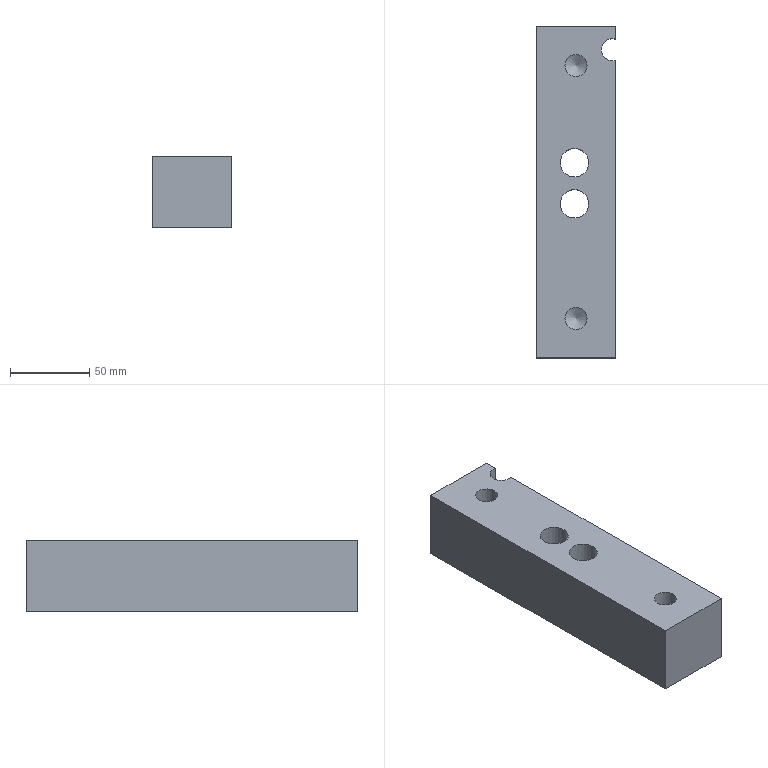Part | STEP file | 012_id2190_x_t | 1 solid | 14 faces | box 50 x 210 x 45 mm | volume 438486 mm3 | plane 7 | cylinder 5 | cone 2 | commonest cylinder face diameters 14 x3 18 x2
STEP:
#1=CARTESIAN_POINT('',(0.,0.,0.));
#2=DIRECTION('',(0.,0.,1.));
#3=DIRECTION('',(1.,0.,0.));
#4=AXIS2_PLACEMENT_3D('',#1,#2,#3);
#5=CARTESIAN_POINT('',(-853.5,103.5,230.));
#6=VERTEX_POINT('',#5);
#7=CARTESIAN_POINT('',(-862.5,103.5,230.));
#8=DIRECTION('',(0.,0.,-1.));
#9=DIRECTION('',(1.,0.,0.));
#10=AXIS2_PLACEMENT_3D('',#7,#8,#9);
#11=CIRCLE('',#10,9.);
#12=CARTESIAN_POINT('',(-681.5,-210.,230.));
#13=DIRECTION('',(0.,0.,1.));
#14=DIRECTION('',(1.,0.,0.));
#15=AXIS2_PLACEMENT_3D('',#12,#13,#14);
#16=PLANE('',#15);
#17=CARTESIAN_POINT('',(-172.,313.5));
#18=CARTESIAN_POINT('',(-172.,297.912));
#19=CARTESIAN_POINT('',(-185.5,305.706));
#20=CARTESIAN_POINT('',(-199.,313.5));
#21=CARTESIAN_POINT('',(-185.5,321.294));
#22=CARTESIAN_POINT('',(-172.,329.088));
#23=CARTESIAN_POINT('',(-172.,313.5));
#24=(BOUNDED_CURVE()B_SPLINE_CURVE(2,(#17,#18,#19,#20,#21,#22,#23),.UNSPECIFIED.,.T.,.F.)B_SPLINE_CURVE_WITH_KNOTS((1,2,2,2,2,1),(-2.094,0.,2.094,4.189,6.283,8.378),.UNSPECIFIED.)CURVE()GEOMETRIC_REPRESENTATION_ITEM()RATIONAL_B_SPLINE_CURVE((1.,0.5,1.,0.5,1.,0.5,1.))REPRESENTATION_ITEM(''));
#25=(GEOMETRIC_REPRESENTATION_CONTEXT(2)PARAMETRIC_REPRESENTATION_CONTEXT()REPRESENTATION_CONTEXT('',''));
#26=DEFINITIONAL_REPRESENTATION('',(#24),#25);
#27=PCURVE('',#16,#26);
#28=CARTESIAN_POINT('',(-862.5,103.5,510.));
#29=DIRECTION('',(0.,0.,-1.));
#30=DIRECTION('',(-1.,0.,0.));
#31=AXIS2_PLACEMENT_3D('',#28,#29,#30);
#32=CYLINDRICAL_SURFACE('',#31,9.);
#33=CARTESIAN_POINT('',(3.142,280.));
#34=DIRECTION('',(1.,0.));
#35=VECTOR('',#34,1.);
#36=LINE('',#33,#35);
#37=(GEOMETRIC_REPRESENTATION_CONTEXT(2)PARAMETRIC_REPRESENTATION_CONTEXT()REPRESENTATION_CONTEXT('',''));
#38=DEFINITIONAL_REPRESENTATION('',(#36),#37);
#39=PCURVE('',#32,#38);
#40=SURFACE_CURVE('',#11,(#27,#39),.PCURVE_S1.);
#41=EDGE_CURVE('',#6,#6,#40,.T.);
#42=ORIENTED_EDGE('',*,*,#41,.T.);
#43=EDGE_LOOP('',(#42));
#44=FACE_BOUND('',#43,.T.);
#45=CARTESIAN_POINT('',(-868.5,165.,230.));
#46=VERTEX_POINT('',#45);
#47=CARTESIAN_POINT('',(-854.5,165.,230.));
#48=VERTEX_POINT('',#47);
#49=CARTESIAN_POINT('',(-861.5,165.,230.));
#50=DIRECTION('',(0.,0.,1.));
#51=DIRECTION('',(-1.,0.,0.));
#52=AXIS2_PLACEMENT_3D('',#49,#50,#51);
#53=CIRCLE('',#52,7.);
#54=CARTESIAN_POINT('',(-180.,375.));
#55=DIRECTION('',(-1.,0.));
#56=AXIS2_PLACEMENT_2D('',#54,#55);
#57=CIRCLE('',#56,7.);
#58=(GEOMETRIC_REPRESENTATION_CONTEXT(2)PARAMETRIC_REPRESENTATION_CONTEXT()REPRESENTATION_CONTEXT('',''));
#59=DEFINITIONAL_REPRESENTATION('',(#57),#58);
#60=PCURVE('',#16,#59);
#61=CARTESIAN_POINT('',(-861.5,165.,279.));
#62=DIRECTION('',(0.,0.,-1.));
#63=DIRECTION('',(1.,0.,0.));
#64=AXIS2_PLACEMENT_3D('',#61,#62,#63);
#65=CYLINDRICAL_SURFACE('',#64,7.);
#66=CARTESIAN_POINT('',(3.142,49.));
#67=DIRECTION('',(-1.,0.));
#68=VECTOR('',#67,1.);
#69=LINE('',#66,#68);
#70=(GEOMETRIC_REPRESENTATION_CONTEXT(2)PARAMETRIC_REPRESENTATION_CONTEXT()REPRESENTATION_CONTEXT('',''));
#71=DEFINITIONAL_REPRESENTATION('',(#69),#70);
#72=PCURVE('',#65,#71);
#73=SURFACE_CURVE('',#53,(#60,#72),.PCURVE_S1.);
#74=EDGE_CURVE('',#46,#48,#73,.T.);
#75=ORIENTED_EDGE('',*,*,#74,.F.);
#76=CARTESIAN_POINT('',(-861.5,165.,230.));
#77=DIRECTION('',(0.,0.,1.));
#78=DIRECTION('',(-1.,0.,0.));
#79=AXIS2_PLACEMENT_3D('',#76,#77,#78);
#80=CIRCLE('',#79,7.);
#81=CARTESIAN_POINT('',(-180.,375.));
#82=DIRECTION('',(-1.,0.));
#83=AXIS2_PLACEMENT_2D('',#81,#82);
#84=CIRCLE('',#83,7.);
#85=(GEOMETRIC_REPRESENTATION_CONTEXT(2)PARAMETRIC_REPRESENTATION_CONTEXT()REPRESENTATION_CONTEXT('',''));
#86=DEFINITIONAL_REPRESENTATION('',(#84),#85);
#87=PCURVE('',#16,#86);
#88=CARTESIAN_POINT('',(9.425,49.));
#89=DIRECTION('',(-1.,0.));
#90=VECTOR('',#89,1.);
#91=LINE('',#88,#90);
#92=(GEOMETRIC_REPRESENTATION_CONTEXT(2)PARAMETRIC_REPRESENTATION_CONTEXT()REPRESENTATION_CONTEXT('',''));
#93=DEFINITIONAL_REPRESENTATION('',(#91),#92);
#94=PCURVE('',#65,#93);
#95=SURFACE_CURVE('',#80,(#87,#94),.PCURVE_S1.);
#96=EDGE_CURVE('',#48,#46,#95,.T.);
#97=ORIENTED_EDGE('',*,*,#96,.F.);
#98=EDGE_LOOP('',(#75,#97));
#99=FACE_BOUND('',#98,.T.);
#100=CARTESIAN_POINT('',(-868.5,5.,230.));
#101=VERTEX_POINT('',#100);
#102=CARTESIAN_POINT('',(-854.5,5.,230.));
#103=VERTEX_POINT('',#102);
#104=CARTESIAN_POINT('',(-861.5,5.,230.));
#105=DIRECTION('',(0.,0.,-1.));
#106=DIRECTION('',(-1.,0.,0.));
#107=AXIS2_PLACEMENT_3D('',#104,#105,#106);
#108=CIRCLE('',#107,7.);
#109=CARTESIAN_POINT('',(-187.,215.));
#110=CARTESIAN_POINT('',(-187.,227.124));
#111=CARTESIAN_POINT('',(-176.5,221.062));
#112=CARTESIAN_POINT('',(-166.,215.));
#113=CARTESIAN_POINT('',(-176.5,208.938));
#114=CARTESIAN_POINT('',(-187.,202.876));
#115=CARTESIAN_POINT('',(-187.,215.));
#116=(BOUNDED_CURVE()B_SPLINE_CURVE(2,(#109,#110,#111,#112,#113,#114,#115),.UNSPECIFIED.,.T.,.F.)B_SPLINE_CURVE_WITH_KNOTS((1,2,2,2,2,1),(-2.094,0.,2.094,4.189,6.283,8.378),.UNSPECIFIED.)CURVE()GEOMETRIC_REPRESENTATION_ITEM()RATIONAL_B_SPLINE_CURVE((1.,0.5,1.,0.5,1.,0.5,1.))REPRESENTATION_ITEM(''));
#117=(GEOMETRIC_REPRESENTATION_CONTEXT(2)PARAMETRIC_REPRESENTATION_CONTEXT()REPRESENTATION_CONTEXT('',''));
#118=DEFINITIONAL_REPRESENTATION('',(#116),#117);
#119=PCURVE('',#16,#118);
#120=CARTESIAN_POINT('',(-861.5,5.,279.));
#121=DIRECTION('',(0.,0.,-1.));
#122=DIRECTION('',(1.,0.,0.));
#123=AXIS2_PLACEMENT_3D('',#120,#121,#122);
#124=CYLINDRICAL_SURFACE('',#123,7.);
#125=CARTESIAN_POINT('',(3.142,49.));
#126=DIRECTION('',(1.,0.));
#127=VECTOR('',#126,1.);
#128=LINE('',#125,#127);
#129=(GEOMETRIC_REPRESENTATION_CONTEXT(2)PARAMETRIC_REPRESENTATION_CONTEXT()REPRESENTATION_CONTEXT('',''));
#130=DEFINITIONAL_REPRESENTATION('',(#128),#129);
#131=PCURVE('',#124,#130);
#132=SURFACE_CURVE('',#108,(#119,#131),.PCURVE_S1.);
#133=EDGE_CURVE('',#101,#103,#132,.T.);
#134=ORIENTED_EDGE('',*,*,#133,.T.);
#135=CARTESIAN_POINT('',(-861.5,5.,230.));
#136=DIRECTION('',(0.,0.,-1.));
#137=DIRECTION('',(-1.,0.,0.));
#138=AXIS2_PLACEMENT_3D('',#135,#136,#137);
#139=CIRCLE('',#138,7.);
#140=CARTESIAN_POINT('',(-187.,215.));
#141=CARTESIAN_POINT('',(-187.,227.124));
#142=CARTESIAN_POINT('',(-176.5,221.062));
#143=CARTESIAN_POINT('',(-166.,215.));
#144=CARTESIAN_POINT('',(-176.5,208.938));
#145=CARTESIAN_POINT('',(-187.,202.876));
#146=CARTESIAN_POINT('',(-187.,215.));
#147=(BOUNDED_CURVE()B_SPLINE_CURVE(2,(#140,#141,#142,#143,#144,#145,#146),.UNSPECIFIED.,.T.,.F.)B_SPLINE_CURVE_WITH_KNOTS((1,2,2,2,2,1),(-2.094,0.,2.094,4.189,6.283,8.378),.UNSPECIFIED.)CURVE()GEOMETRIC_REPRESENTATION_ITEM()RATIONAL_B_SPLINE_CURVE((1.,0.5,1.,0.5,1.,0.5,1.))REPRESENTATION_ITEM(''));
#148=(GEOMETRIC_REPRESENTATION_CONTEXT(2)PARAMETRIC_REPRESENTATION_CONTEXT()REPRESENTATION_CONTEXT('',''));
#149=DEFINITIONAL_REPRESENTATION('',(#147),#148);
#150=PCURVE('',#16,#149);
#151=CARTESIAN_POINT('',(-3.142,49.));
#152=DIRECTION('',(1.,0.));
#153=VECTOR('',#152,1.);
#154=LINE('',#151,#153);
#155=(GEOMETRIC_REPRESENTATION_CONTEXT(2)PARAMETRIC_REPRESENTATION_CONTEXT()REPRESENTATION_CONTEXT('',''));
#156=DEFINITIONAL_REPRESENTATION('',(#154),#155);
#157=PCURVE('',#124,#156);
#158=SURFACE_CURVE('',#139,(#150,#157),.PCURVE_S1.);
#159=EDGE_CURVE('',#103,#101,#158,.T.);
#160=ORIENTED_EDGE('',*,*,#159,.T.);
#161=EDGE_LOOP('',(#134,#160));
#162=FACE_BOUND('',#161,.T.);
#163=CARTESIAN_POINT('',(-853.5,77.5,230.));
#164=VERTEX_POINT('',#163);
#165=CARTESIAN_POINT('',(-862.5,77.5,230.));
#166=DIRECTION('',(0.,0.,1.));
#167=DIRECTION('',(1.,0.,0.));
#168=AXIS2_PLACEMENT_3D('',#165,#166,#167);
#169=CIRCLE('',#168,9.);
#170=CARTESIAN_POINT('',(-181.,287.5));
#171=DIRECTION('',(1.,0.));
#172=AXIS2_PLACEMENT_2D('',#170,#171);
#173=CIRCLE('',#172,9.);
#174=(GEOMETRIC_REPRESENTATION_CONTEXT(2)PARAMETRIC_REPRESENTATION_CONTEXT()REPRESENTATION_CONTEXT('',''));
#175=DEFINITIONAL_REPRESENTATION('',(#173),#174);
#176=PCURVE('',#16,#175);
#177=CARTESIAN_POINT('',(-862.5,77.5,510.));
#178=DIRECTION('',(0.,0.,-1.));
#179=DIRECTION('',(-1.,0.,0.));
#180=AXIS2_PLACEMENT_3D('',#177,#178,#179);
#181=CYLINDRICAL_SURFACE('',#180,9.);
#182=CARTESIAN_POINT('',(9.425,280.));
#183=DIRECTION('',(-1.,0.));
#184=VECTOR('',#183,1.);
#185=LINE('',#182,#184);
#186=(GEOMETRIC_REPRESENTATION_CONTEXT(2)PARAMETRIC_REPRESENTATION_CONTEXT()REPRESENTATION_CONTEXT('',''));
#187=DEFINITIONAL_REPRESENTATION('',(#185),#186);
#188=PCURVE('',#181,#187);
#189=SURFACE_CURVE('',#169,(#176,#188),.PCURVE_S1.);
#190=EDGE_CURVE('',#164,#164,#189,.T.);
#191=ORIENTED_EDGE('',*,*,#190,.F.);
#192=EDGE_LOOP('',(#191));
#193=FACE_BOUND('',#192,.T.);
#194=CARTESIAN_POINT('',(-836.5,-20.,230.));
#195=VERTEX_POINT('',#194);
#196=CARTESIAN_POINT('',(-836.5,168.292,230.));
#197=VERTEX_POINT('',#196);
#198=CARTESIAN_POINT('',(-836.5,-420.,230.));
#199=DIRECTION('',(0.,1.,0.));
#200=VECTOR('',#199,1.);
#201=LINE('',#198,#200);
#202=CARTESIAN_POINT('',(-155.,-210.));
#203=DIRECTION('',(0.,1.));
#204=VECTOR('',#203,1.);
#205=LINE('',#202,#204);
#206=(GEOMETRIC_REPRESENTATION_CONTEXT(2)PARAMETRIC_REPRESENTATION_CONTEXT()REPRESENTATION_CONTEXT('',''));
#207=DEFINITIONAL_REPRESENTATION('',(#205),#206);
#208=PCURVE('',#16,#207);
#209=CARTESIAN_POINT('',(-836.5,-420.,428.5));
#210=DIRECTION('',(-1.,0.,0.));
#211=DIRECTION('',(0.,0.,-1.));
#212=AXIS2_PLACEMENT_3D('',#209,#210,#211);
#213=PLANE('',#212);
#214=CARTESIAN_POINT('',(198.5,0.));
#215=DIRECTION('',(0.,-1.));
#216=VECTOR('',#215,1.);
#217=LINE('',#214,#216);
#218=(GEOMETRIC_REPRESENTATION_CONTEXT(2)PARAMETRIC_REPRESENTATION_CONTEXT()REPRESENTATION_CONTEXT('',''));
#219=DEFINITIONAL_REPRESENTATION('',(#217),#218);
#220=PCURVE('',#213,#219);
#221=SURFACE_CURVE('',#201,(#208,#220),.PCURVE_S1.);
#222=EDGE_CURVE('',#195,#197,#221,.T.);
#223=ORIENTED_EDGE('',*,*,#222,.T.);
#224=CARTESIAN_POINT('',(-836.5,181.708,230.));
#225=VERTEX_POINT('',#224);
#226=CARTESIAN_POINT('',(-838.5,175.,230.));
#227=DIRECTION('',(0.,0.,-1.));
#228=DIRECTION('',(1.,0.,0.));
#229=AXIS2_PLACEMENT_3D('',#226,#227,#228);
#230=CIRCLE('',#229,7.);
#231=CARTESIAN_POINT('',(-150.,385.));
#232=CARTESIAN_POINT('',(-150.,372.876));
#233=CARTESIAN_POINT('',(-160.5,378.938));
#234=CARTESIAN_POINT('',(-171.,385.));
#235=CARTESIAN_POINT('',(-160.5,391.062));
#236=CARTESIAN_POINT('',(-150.,397.124));
#237=CARTESIAN_POINT('',(-150.,385.));
#238=(BOUNDED_CURVE()B_SPLINE_CURVE(2,(#231,#232,#233,#234,#235,#236,#237),.UNSPECIFIED.,.T.,.F.)B_SPLINE_CURVE_WITH_KNOTS((1,2,2,2,2,1),(-2.094,0.,2.094,4.189,6.283,8.378),.UNSPECIFIED.)CURVE()GEOMETRIC_REPRESENTATION_ITEM()RATIONAL_B_SPLINE_CURVE((1.,0.5,1.,0.5,1.,0.5,1.))REPRESENTATION_ITEM(''));
#239=(GEOMETRIC_REPRESENTATION_CONTEXT(2)PARAMETRIC_REPRESENTATION_CONTEXT()REPRESENTATION_CONTEXT('',''));
#240=DEFINITIONAL_REPRESENTATION('',(#238),#239);
#241=PCURVE('',#16,#240);
#242=CARTESIAN_POINT('',(-838.5,175.,595.));
#243=DIRECTION('',(0.,0.,-1.));
#244=DIRECTION('',(-1.,0.,0.));
#245=AXIS2_PLACEMENT_3D('',#242,#243,#244);
#246=CYLINDRICAL_SURFACE('',#245,7.);
#247=CARTESIAN_POINT('',(-3.142,365.));
#248=DIRECTION('',(1.,0.));
#249=VECTOR('',#248,1.);
#250=LINE('',#247,#249);
#251=(GEOMETRIC_REPRESENTATION_CONTEXT(2)PARAMETRIC_REPRESENTATION_CONTEXT()REPRESENTATION_CONTEXT('',''));
#252=DEFINITIONAL_REPRESENTATION('',(#250),#251);
#253=PCURVE('',#246,#252);
#254=SURFACE_CURVE('',#230,(#241,#253),.PCURVE_S1.);
#255=EDGE_CURVE('',#197,#225,#254,.T.);
#256=ORIENTED_EDGE('',*,*,#255,.T.);
#257=CARTESIAN_POINT('',(-836.5,190.,230.));
#258=VERTEX_POINT('',#257);
#259=CARTESIAN_POINT('',(-836.5,-420.,230.));
#260=DIRECTION('',(0.,1.,0.));
#261=VECTOR('',#260,1.);
#262=LINE('',#259,#261);
#263=CARTESIAN_POINT('',(-155.,-210.));
#264=DIRECTION('',(0.,1.));
#265=VECTOR('',#264,1.);
#266=LINE('',#263,#265);
#267=(GEOMETRIC_REPRESENTATION_CONTEXT(2)PARAMETRIC_REPRESENTATION_CONTEXT()REPRESENTATION_CONTEXT('',''));
#268=DEFINITIONAL_REPRESENTATION('',(#266),#267);
#269=PCURVE('',#16,#268);
#270=CARTESIAN_POINT('',(-836.5,-420.,428.5));
#271=DIRECTION('',(-1.,0.,0.));
#272=DIRECTION('',(0.,0.,-1.));
#273=AXIS2_PLACEMENT_3D('',#270,#271,#272);
#274=PLANE('',#273);
#275=CARTESIAN_POINT('',(198.5,0.));
#276=DIRECTION('',(0.,-1.));
#277=VECTOR('',#276,1.);
#278=LINE('',#275,#277);
#279=(GEOMETRIC_REPRESENTATION_CONTEXT(2)PARAMETRIC_REPRESENTATION_CONTEXT()REPRESENTATION_CONTEXT('',''));
#280=DEFINITIONAL_REPRESENTATION('',(#278),#279);
#281=PCURVE('',#274,#280);
#282=SURFACE_CURVE('',#262,(#269,#281),.PCURVE_S1.);
#283=EDGE_CURVE('',#225,#258,#282,.T.);
#284=ORIENTED_EDGE('',*,*,#283,.T.);
#285=CARTESIAN_POINT('',(-886.5,190.,230.));
#286=VERTEX_POINT('',#285);
#287=CARTESIAN_POINT('',(-886.5,190.,230.));
#288=DIRECTION('',(-1.,0.,0.));
#289=VECTOR('',#288,1.);
#290=LINE('',#287,#289);
#291=CARTESIAN_POINT('',(-205.,400.));
#292=DIRECTION('',(-1.,0.));
#293=VECTOR('',#292,1.);
#294=LINE('',#291,#293);
#295=(GEOMETRIC_REPRESENTATION_CONTEXT(2)PARAMETRIC_REPRESENTATION_CONTEXT()REPRESENTATION_CONTEXT('',''));
#296=DEFINITIONAL_REPRESENTATION('',(#294),#295);
#297=PCURVE('',#16,#296);
#298=CARTESIAN_POINT('',(-886.5,190.,428.5));
#299=DIRECTION('',(0.,1.,0.));
#300=DIRECTION('',(0.,0.,1.));
#301=AXIS2_PLACEMENT_3D('',#298,#299,#300);
#302=PLANE('',#301);
#303=CARTESIAN_POINT('',(-198.5,0.));
#304=DIRECTION('',(0.,-1.));
#305=VECTOR('',#304,1.);
#306=LINE('',#303,#305);
#307=(GEOMETRIC_REPRESENTATION_CONTEXT(2)PARAMETRIC_REPRESENTATION_CONTEXT()REPRESENTATION_CONTEXT('',''));
#308=DEFINITIONAL_REPRESENTATION('',(#306),#307);
#309=PCURVE('',#302,#308);
#310=SURFACE_CURVE('',#290,(#297,#309),.PCURVE_S1.);
#311=EDGE_CURVE('',#258,#286,#310,.T.);
#312=ORIENTED_EDGE('',*,*,#311,.T.);
#313=CARTESIAN_POINT('',(-886.5,-20.,230.));
#314=VERTEX_POINT('',#313);
#315=CARTESIAN_POINT('',(-886.5,-420.,230.));
#316=DIRECTION('',(0.,-1.,0.));
#317=VECTOR('',#316,1.);
#318=LINE('',#315,#317);
#319=CARTESIAN_POINT('',(-205.,-210.));
#320=DIRECTION('',(0.,-1.));
#321=VECTOR('',#320,1.);
#322=LINE('',#319,#321);
#323=(GEOMETRIC_REPRESENTATION_CONTEXT(2)PARAMETRIC_REPRESENTATION_CONTEXT()REPRESENTATION_CONTEXT('',''));
#324=DEFINITIONAL_REPRESENTATION('',(#322),#323);
#325=PCURVE('',#16,#324);
#326=CARTESIAN_POINT('',(-886.5,-420.,428.5));
#327=DIRECTION('',(-1.,0.,0.));
#328=DIRECTION('',(0.,0.,-1.));
#329=AXIS2_PLACEMENT_3D('',#326,#327,#328);
#330=PLANE('',#329);
#331=CARTESIAN_POINT('',(198.5,0.));
#332=DIRECTION('',(0.,1.));
#333=VECTOR('',#332,1.);
#334=LINE('',#331,#333);
#335=(GEOMETRIC_REPRESENTATION_CONTEXT(2)PARAMETRIC_REPRESENTATION_CONTEXT()REPRESENTATION_CONTEXT('',''));
#336=DEFINITIONAL_REPRESENTATION('',(#334),#335);
#337=PCURVE('',#330,#336);
#338=SURFACE_CURVE('',#318,(#325,#337),.PCURVE_S1.);
#339=EDGE_CURVE('',#286,#314,#338,.T.);
#340=ORIENTED_EDGE('',*,*,#339,.T.);
#341=CARTESIAN_POINT('',(-886.5,-20.,230.));
#342=DIRECTION('',(-1.,0.,0.));
#343=VECTOR('',#342,1.);
#344=LINE('',#341,#343);
#345=CARTESIAN_POINT('',(-205.,190.));
#346=DIRECTION('',(-1.,0.));
#347=VECTOR('',#346,1.);
#348=LINE('',#345,#347);
#349=(GEOMETRIC_REPRESENTATION_CONTEXT(2)PARAMETRIC_REPRESENTATION_CONTEXT()REPRESENTATION_CONTEXT('',''));
#350=DEFINITIONAL_REPRESENTATION('',(#348),#349);
#351=PCURVE('',#16,#350);
#352=CARTESIAN_POINT('',(-886.5,-20.,428.5));
#353=DIRECTION('',(0.,1.,0.));
#354=DIRECTION('',(0.,0.,1.));
#355=AXIS2_PLACEMENT_3D('',#352,#353,#354);
#356=PLANE('',#355);
#357=CARTESIAN_POINT('',(-198.5,0.));
#358=DIRECTION('',(0.,-1.));
#359=VECTOR('',#358,1.);
#360=LINE('',#357,#359);
#361=(GEOMETRIC_REPRESENTATION_CONTEXT(2)PARAMETRIC_REPRESENTATION_CONTEXT()REPRESENTATION_CONTEXT('',''));
#362=DEFINITIONAL_REPRESENTATION('',(#360),#361);
#363=PCURVE('',#356,#362);
#364=SURFACE_CURVE('',#344,(#351,#363),.PCURVE_S1.);
#365=EDGE_CURVE('',#195,#314,#364,.T.);
#366=ORIENTED_EDGE('',*,*,#365,.F.);
#367=EDGE_LOOP('',(#223,#256,#284,#312,#340,#366));
#368=FACE_BOUND('',#367,.T.);
#369=ADVANCED_FACE('',(#44,#99,#162,#193,#368),#16,.T.);
#370=CARTESIAN_POINT('',(-836.5,181.708,185.));
#371=VERTEX_POINT('',#370);
#372=CARTESIAN_POINT('',(-836.5,181.708,595.));
#373=DIRECTION('',(0.,0.,1.));
#374=VECTOR('',#373,1.);
#375=LINE('',#372,#374);
#376=CARTESIAN_POINT('',(-166.5,-601.708));
#377=DIRECTION('',(-1.,0.));
#378=VECTOR('',#377,1.);
#379=LINE('',#376,#378);
#380=(GEOMETRIC_REPRESENTATION_CONTEXT(2)PARAMETRIC_REPRESENTATION_CONTEXT()REPRESENTATION_CONTEXT('',''));
#381=DEFINITIONAL_REPRESENTATION('',(#379),#380);
#382=PCURVE('',#274,#381);
#383=CARTESIAN_POINT('',(1.861,0.));
#384=DIRECTION('',(0.,-1.));
#385=VECTOR('',#384,1.);
#386=LINE('',#383,#385);
#387=(GEOMETRIC_REPRESENTATION_CONTEXT(2)PARAMETRIC_REPRESENTATION_CONTEXT()REPRESENTATION_CONTEXT('',''));
#388=DEFINITIONAL_REPRESENTATION('',(#386),#387);
#389=PCURVE('',#246,#388);
#390=SURFACE_CURVE('',#375,(#382,#389),.PCURVE_S1.);
#391=EDGE_CURVE('',#371,#225,#390,.T.);
#392=ORIENTED_EDGE('',*,*,#391,.F.);
#393=CARTESIAN_POINT('',(-836.5,190.,185.));
#394=VERTEX_POINT('',#393);
#395=CARTESIAN_POINT('',(-836.5,-420.,185.));
#396=DIRECTION('',(0.,1.,0.));
#397=VECTOR('',#396,1.);
#398=LINE('',#395,#397);
#399=CARTESIAN_POINT('',(243.5,0.));
#400=DIRECTION('',(0.,-1.));
#401=VECTOR('',#400,1.);
#402=LINE('',#399,#401);
#403=(GEOMETRIC_REPRESENTATION_CONTEXT(2)PARAMETRIC_REPRESENTATION_CONTEXT()REPRESENTATION_CONTEXT('',''));
#404=DEFINITIONAL_REPRESENTATION('',(#402),#403);
#405=PCURVE('',#274,#404);
#406=CARTESIAN_POINT('',(-886.5,-420.,185.));
#407=DIRECTION('',(0.,0.,1.));
#408=DIRECTION('',(0.,-1.,0.));
#409=AXIS2_PLACEMENT_3D('',#406,#407,#408);
#410=PLANE('',#409);
#411=CARTESIAN_POINT('',(0.,50.));
#412=DIRECTION('',(-1.,0.));
#413=VECTOR('',#412,1.);
#414=LINE('',#411,#413);
#415=(GEOMETRIC_REPRESENTATION_CONTEXT(2)PARAMETRIC_REPRESENTATION_CONTEXT()REPRESENTATION_CONTEXT('',''));
#416=DEFINITIONAL_REPRESENTATION('',(#414),#415);
#417=PCURVE('',#410,#416);
#418=SURFACE_CURVE('',#398,(#405,#417),.PCURVE_S1.);
#419=EDGE_CURVE('',#371,#394,#418,.T.);
#420=ORIENTED_EDGE('',*,*,#419,.T.);
#421=CARTESIAN_POINT('',(-836.5,190.,428.5));
#422=DIRECTION('',(0.,0.,1.));
#423=VECTOR('',#422,1.);
#424=LINE('',#421,#423);
#425=CARTESIAN_POINT('',(0.,-610.));
#426=DIRECTION('',(-1.,0.));
#427=VECTOR('',#426,1.);
#428=LINE('',#425,#427);
#429=(GEOMETRIC_REPRESENTATION_CONTEXT(2)PARAMETRIC_REPRESENTATION_CONTEXT()REPRESENTATION_CONTEXT('',''));
#430=DEFINITIONAL_REPRESENTATION('',(#428),#429);
#431=PCURVE('',#274,#430);
#432=CARTESIAN_POINT('',(0.,50.));
#433=DIRECTION('',(1.,0.));
#434=VECTOR('',#433,1.);
#435=LINE('',#432,#434);
#436=(GEOMETRIC_REPRESENTATION_CONTEXT(2)PARAMETRIC_REPRESENTATION_CONTEXT()REPRESENTATION_CONTEXT('',''));
#437=DEFINITIONAL_REPRESENTATION('',(#435),#436);
#438=PCURVE('',#302,#437);
#439=SURFACE_CURVE('',#424,(#431,#438),.PCURVE_S1.);
#440=EDGE_CURVE('',#394,#258,#439,.T.);
#441=ORIENTED_EDGE('',*,*,#440,.T.);
#442=ORIENTED_EDGE('',*,*,#283,.F.);
#443=EDGE_LOOP('',(#392,#420,#441,#442));
#444=FACE_BOUND('',#443,.T.);
#445=ADVANCED_FACE('',(#444),#274,.F.);
#446=CARTESIAN_POINT('',(-836.5,168.292,185.));
#447=VERTEX_POINT('',#446);
#448=CARTESIAN_POINT('',(-836.5,168.292,595.));
#449=DIRECTION('',(0.,0.,-1.));
#450=VECTOR('',#449,1.);
#451=LINE('',#448,#450);
#452=CARTESIAN_POINT('',(-166.5,-588.292));
#453=DIRECTION('',(1.,0.));
#454=VECTOR('',#453,1.);
#455=LINE('',#452,#454);
#456=(GEOMETRIC_REPRESENTATION_CONTEXT(2)PARAMETRIC_REPRESENTATION_CONTEXT()REPRESENTATION_CONTEXT('',''));
#457=DEFINITIONAL_REPRESENTATION('',(#455),#456);
#458=PCURVE('',#213,#457);
#459=CARTESIAN_POINT('',(-1.861,0.));
#460=DIRECTION('',(0.,1.));
#461=VECTOR('',#460,1.);
#462=LINE('',#459,#461);
#463=(GEOMETRIC_REPRESENTATION_CONTEXT(2)PARAMETRIC_REPRESENTATION_CONTEXT()REPRESENTATION_CONTEXT('',''));
#464=DEFINITIONAL_REPRESENTATION('',(#462),#463);
#465=PCURVE('',#246,#464);
#466=SURFACE_CURVE('',#451,(#458,#465),.PCURVE_S1.);
#467=EDGE_CURVE('',#197,#447,#466,.T.);
#468=ORIENTED_EDGE('',*,*,#467,.F.);
#469=ORIENTED_EDGE('',*,*,#222,.F.);
#470=CARTESIAN_POINT('',(-836.5,-20.,185.));
#471=VERTEX_POINT('',#470);
#472=CARTESIAN_POINT('',(-836.5,-20.,428.5));
#473=DIRECTION('',(0.,0.,-1.));
#474=VECTOR('',#473,1.);
#475=LINE('',#472,#474);
#476=CARTESIAN_POINT('',(0.,-400.));
#477=DIRECTION('',(1.,0.));
#478=VECTOR('',#477,1.);
#479=LINE('',#476,#478);
#480=(GEOMETRIC_REPRESENTATION_CONTEXT(2)PARAMETRIC_REPRESENTATION_CONTEXT()REPRESENTATION_CONTEXT('',''));
#481=DEFINITIONAL_REPRESENTATION('',(#479),#480);
#482=PCURVE('',#213,#481);
#483=CARTESIAN_POINT('',(0.,50.));
#484=DIRECTION('',(-1.,0.));
#485=VECTOR('',#484,1.);
#486=LINE('',#483,#485);
#487=(GEOMETRIC_REPRESENTATION_CONTEXT(2)PARAMETRIC_REPRESENTATION_CONTEXT()REPRESENTATION_CONTEXT('',''));
#488=DEFINITIONAL_REPRESENTATION('',(#486),#487);
#489=PCURVE('',#356,#488);
#490=SURFACE_CURVE('',#475,(#482,#489),.PCURVE_S1.);
#491=EDGE_CURVE('',#195,#471,#490,.T.);
#492=ORIENTED_EDGE('',*,*,#491,.T.);
#493=CARTESIAN_POINT('',(-836.5,-420.,185.));
#494=DIRECTION('',(0.,1.,0.));
#495=VECTOR('',#494,1.);
#496=LINE('',#493,#495);
#497=CARTESIAN_POINT('',(243.5,0.));
#498=DIRECTION('',(0.,-1.));
#499=VECTOR('',#498,1.);
#500=LINE('',#497,#499);
#501=(GEOMETRIC_REPRESENTATION_CONTEXT(2)PARAMETRIC_REPRESENTATION_CONTEXT()REPRESENTATION_CONTEXT('',''));
#502=DEFINITIONAL_REPRESENTATION('',(#500),#501);
#503=PCURVE('',#213,#502);
#504=CARTESIAN_POINT('',(0.,50.));
#505=DIRECTION('',(-1.,0.));
#506=VECTOR('',#505,1.);
#507=LINE('',#504,#506);
#508=(GEOMETRIC_REPRESENTATION_CONTEXT(2)PARAMETRIC_REPRESENTATION_CONTEXT()REPRESENTATION_CONTEXT('',''));
#509=DEFINITIONAL_REPRESENTATION('',(#507),#508);
#510=PCURVE('',#410,#509);
#511=SURFACE_CURVE('',#496,(#503,#510),.PCURVE_S1.);
#512=EDGE_CURVE('',#471,#447,#511,.T.);
#513=ORIENTED_EDGE('',*,*,#512,.T.);
#514=EDGE_LOOP('',(#468,#469,#492,#513));
#515=FACE_BOUND('',#514,.T.);
#516=ADVANCED_FACE('',(#515),#213,.F.);
#517=ORIENTED_EDGE('',*,*,#419,.F.);
#518=CARTESIAN_POINT('',(-838.5,175.,185.));
#519=DIRECTION('',(0.,0.,1.));
#520=DIRECTION('',(1.,0.,0.));
#521=AXIS2_PLACEMENT_3D('',#518,#519,#520);
#522=CIRCLE('',#521,7.);
#523=CARTESIAN_POINT('',(-595.,48.));
#524=DIRECTION('',(0.,1.));
#525=AXIS2_PLACEMENT_2D('',#523,#524);
#526=CIRCLE('',#525,7.);
#527=(GEOMETRIC_REPRESENTATION_CONTEXT(2)PARAMETRIC_REPRESENTATION_CONTEXT()REPRESENTATION_CONTEXT('',''));
#528=DEFINITIONAL_REPRESENTATION('',(#526),#527);
#529=PCURVE('',#410,#528);
#530=CARTESIAN_POINT('',(3.142,410.));
#531=DIRECTION('',(-1.,0.));
#532=VECTOR('',#531,1.);
#533=LINE('',#530,#532);
#534=(GEOMETRIC_REPRESENTATION_CONTEXT(2)PARAMETRIC_REPRESENTATION_CONTEXT()REPRESENTATION_CONTEXT('',''));
#535=DEFINITIONAL_REPRESENTATION('',(#533),#534);
#536=PCURVE('',#246,#535);
#537=SURFACE_CURVE('',#522,(#529,#536),.PCURVE_S1.);
#538=EDGE_CURVE('',#371,#447,#537,.T.);
#539=ORIENTED_EDGE('',*,*,#538,.T.);
#540=ORIENTED_EDGE('',*,*,#512,.F.);
#541=CARTESIAN_POINT('',(-886.5,-20.,185.));
#542=VERTEX_POINT('',#541);
#543=CARTESIAN_POINT('',(-886.5,-20.,185.));
#544=DIRECTION('',(-1.,0.,0.));
#545=VECTOR('',#544,1.);
#546=LINE('',#543,#545);
#547=CARTESIAN_POINT('',(-400.,0.));
#548=DIRECTION('',(0.,-1.));
#549=VECTOR('',#548,1.);
#550=LINE('',#547,#549);
#551=(GEOMETRIC_REPRESENTATION_CONTEXT(2)PARAMETRIC_REPRESENTATION_CONTEXT()REPRESENTATION_CONTEXT('',''));
#552=DEFINITIONAL_REPRESENTATION('',(#550),#551);
#553=PCURVE('',#410,#552);
#554=CARTESIAN_POINT('',(-243.5,0.));
#555=DIRECTION('',(0.,-1.));
#556=VECTOR('',#555,1.);
#557=LINE('',#554,#556);
#558=(GEOMETRIC_REPRESENTATION_CONTEXT(2)PARAMETRIC_REPRESENTATION_CONTEXT()REPRESENTATION_CONTEXT('',''));
#559=DEFINITIONAL_REPRESENTATION('',(#557),#558);
#560=PCURVE('',#356,#559);
#561=SURFACE_CURVE('',#546,(#553,#560),.PCURVE_S1.);
#562=EDGE_CURVE('',#471,#542,#561,.T.);
#563=ORIENTED_EDGE('',*,*,#562,.T.);
#564=CARTESIAN_POINT('',(-886.5,190.,185.));
#565=VERTEX_POINT('',#564);
#566=CARTESIAN_POINT('',(-886.5,-420.,185.));
#567=DIRECTION('',(0.,1.,0.));
#568=VECTOR('',#567,1.);
#569=LINE('',#566,#568);
#570=CARTESIAN_POINT('',(0.,0.));
#571=DIRECTION('',(-1.,0.));
#572=VECTOR('',#571,1.);
#573=LINE('',#570,#572);
#574=(GEOMETRIC_REPRESENTATION_CONTEXT(2)PARAMETRIC_REPRESENTATION_CONTEXT()REPRESENTATION_CONTEXT('',''));
#575=DEFINITIONAL_REPRESENTATION('',(#573),#574);
#576=PCURVE('',#410,#575);
#577=CARTESIAN_POINT('',(243.5,0.));
#578=DIRECTION('',(0.,-1.));
#579=VECTOR('',#578,1.);
#580=LINE('',#577,#579);
#581=(GEOMETRIC_REPRESENTATION_CONTEXT(2)PARAMETRIC_REPRESENTATION_CONTEXT()REPRESENTATION_CONTEXT('',''));
#582=DEFINITIONAL_REPRESENTATION('',(#580),#581);
#583=PCURVE('',#330,#582);
#584=SURFACE_CURVE('',#569,(#576,#583),.PCURVE_S1.);
#585=EDGE_CURVE('',#542,#565,#584,.T.);
#586=ORIENTED_EDGE('',*,*,#585,.T.);
#587=CARTESIAN_POINT('',(-886.5,190.,185.));
#588=DIRECTION('',(-1.,0.,0.));
#589=VECTOR('',#588,1.);
#590=LINE('',#587,#589);
#591=CARTESIAN_POINT('',(-610.,0.));
#592=DIRECTION('',(0.,-1.));
#593=VECTOR('',#592,1.);
#594=LINE('',#591,#593);
#595=(GEOMETRIC_REPRESENTATION_CONTEXT(2)PARAMETRIC_REPRESENTATION_CONTEXT()REPRESENTATION_CONTEXT('',''));
#596=DEFINITIONAL_REPRESENTATION('',(#594),#595);
#597=PCURVE('',#410,#596);
#598=CARTESIAN_POINT('',(-243.5,0.));
#599=DIRECTION('',(0.,-1.));
#600=VECTOR('',#599,1.);
#601=LINE('',#598,#600);
#602=(GEOMETRIC_REPRESENTATION_CONTEXT(2)PARAMETRIC_REPRESENTATION_CONTEXT()REPRESENTATION_CONTEXT('',''));
#603=DEFINITIONAL_REPRESENTATION('',(#601),#602);
#604=PCURVE('',#302,#603);
#605=SURFACE_CURVE('',#590,(#597,#604),.PCURVE_S1.);
#606=EDGE_CURVE('',#394,#565,#605,.T.);
#607=ORIENTED_EDGE('',*,*,#606,.F.);
#608=EDGE_LOOP('',(#517,#539,#540,#563,#586,#607));
#609=FACE_BOUND('',#608,.T.);
#610=CARTESIAN_POINT('',(-853.5,77.5,185.));
#611=VERTEX_POINT('',#610);
#612=CARTESIAN_POINT('',(-862.5,77.5,185.));
#613=DIRECTION('',(0.,0.,1.));
#614=DIRECTION('',(1.,0.,0.));
#615=AXIS2_PLACEMENT_3D('',#612,#613,#614);
#616=CIRCLE('',#615,9.);
#617=CARTESIAN_POINT('',(-497.5,24.));
#618=DIRECTION('',(0.,1.));
#619=AXIS2_PLACEMENT_2D('',#617,#618);
#620=CIRCLE('',#619,9.);
#621=(GEOMETRIC_REPRESENTATION_CONTEXT(2)PARAMETRIC_REPRESENTATION_CONTEXT()REPRESENTATION_CONTEXT('',''));
#622=DEFINITIONAL_REPRESENTATION('',(#620),#621);
#623=PCURVE('',#410,#622);
#624=CARTESIAN_POINT('',(9.425,325.));
#625=DIRECTION('',(-1.,0.));
#626=VECTOR('',#625,1.);
#627=LINE('',#624,#626);
#628=(GEOMETRIC_REPRESENTATION_CONTEXT(2)PARAMETRIC_REPRESENTATION_CONTEXT()REPRESENTATION_CONTEXT('',''));
#629=DEFINITIONAL_REPRESENTATION('',(#627),#628);
#630=PCURVE('',#181,#629);
#631=SURFACE_CURVE('',#616,(#623,#630),.PCURVE_S1.);
#632=EDGE_CURVE('',#611,#611,#631,.T.);
#633=ORIENTED_EDGE('',*,*,#632,.T.);
#634=EDGE_LOOP('',(#633));
#635=FACE_BOUND('',#634,.T.);
#636=CARTESIAN_POINT('',(-853.5,103.5,185.));
#637=VERTEX_POINT('',#636);
#638=CARTESIAN_POINT('',(-862.5,103.5,185.));
#639=DIRECTION('',(0.,0.,-1.));
#640=DIRECTION('',(1.,0.,0.));
#641=AXIS2_PLACEMENT_3D('',#638,#639,#640);
#642=CIRCLE('',#641,9.);
#643=CARTESIAN_POINT('',(-523.5,33.));
#644=CARTESIAN_POINT('',(-507.912,33.));
#645=CARTESIAN_POINT('',(-515.706,19.5));
#646=CARTESIAN_POINT('',(-523.5,6.));
#647=CARTESIAN_POINT('',(-531.294,19.5));
#648=CARTESIAN_POINT('',(-539.088,33.));
#649=CARTESIAN_POINT('',(-523.5,33.));
#650=(BOUNDED_CURVE()B_SPLINE_CURVE(2,(#643,#644,#645,#646,#647,#648,#649),.UNSPECIFIED.,.T.,.F.)B_SPLINE_CURVE_WITH_KNOTS((1,2,2,2,2,1),(-2.094,0.,2.094,4.189,6.283,8.378),.UNSPECIFIED.)CURVE()GEOMETRIC_REPRESENTATION_ITEM()RATIONAL_B_SPLINE_CURVE((1.,0.5,1.,0.5,1.,0.5,1.))REPRESENTATION_ITEM(''));
#651=(GEOMETRIC_REPRESENTATION_CONTEXT(2)PARAMETRIC_REPRESENTATION_CONTEXT()REPRESENTATION_CONTEXT('',''));
#652=DEFINITIONAL_REPRESENTATION('',(#650),#651);
#653=PCURVE('',#410,#652);
#654=CARTESIAN_POINT('',(3.142,325.));
#655=DIRECTION('',(1.,0.));
#656=VECTOR('',#655,1.);
#657=LINE('',#654,#656);
#658=(GEOMETRIC_REPRESENTATION_CONTEXT(2)PARAMETRIC_REPRESENTATION_CONTEXT()REPRESENTATION_CONTEXT('',''));
#659=DEFINITIONAL_REPRESENTATION('',(#657),#658);
#660=PCURVE('',#32,#659);
#661=SURFACE_CURVE('',#642,(#653,#660),.PCURVE_S1.);
#662=EDGE_CURVE('',#637,#637,#661,.T.);
#663=ORIENTED_EDGE('',*,*,#662,.F.);
#664=EDGE_LOOP('',(#663));
#665=FACE_BOUND('',#664,.T.);
#666=ADVANCED_FACE('',(#609,#635,#665),#410,.F.);
#667=ORIENTED_EDGE('',*,*,#365,.T.);
#668=CARTESIAN_POINT('',(-886.5,-20.,428.5));
#669=DIRECTION('',(0.,0.,-1.));
#670=VECTOR('',#669,1.);
#671=LINE('',#668,#670);
#672=CARTESIAN_POINT('',(0.,0.));
#673=DIRECTION('',(-1.,0.));
#674=VECTOR('',#673,1.);
#675=LINE('',#672,#674);
#676=(GEOMETRIC_REPRESENTATION_CONTEXT(2)PARAMETRIC_REPRESENTATION_CONTEXT()REPRESENTATION_CONTEXT('',''));
#677=DEFINITIONAL_REPRESENTATION('',(#675),#676);
#678=PCURVE('',#356,#677);
#679=CARTESIAN_POINT('',(0.,-400.));
#680=DIRECTION('',(1.,0.));
#681=VECTOR('',#680,1.);
#682=LINE('',#679,#681);
#683=(GEOMETRIC_REPRESENTATION_CONTEXT(2)PARAMETRIC_REPRESENTATION_CONTEXT()REPRESENTATION_CONTEXT('',''));
#684=DEFINITIONAL_REPRESENTATION('',(#682),#683);
#685=PCURVE('',#330,#684);
#686=SURFACE_CURVE('',#671,(#678,#685),.PCURVE_S1.);
#687=EDGE_CURVE('',#314,#542,#686,.T.);
#688=ORIENTED_EDGE('',*,*,#687,.T.);
#689=ORIENTED_EDGE('',*,*,#562,.F.);
#690=ORIENTED_EDGE('',*,*,#491,.F.);
#691=EDGE_LOOP('',(#667,#688,#689,#690));
#692=FACE_BOUND('',#691,.T.);
#693=ADVANCED_FACE('',(#692),#356,.F.);
#694=CARTESIAN_POINT('',(-886.5,190.,428.5));
#695=DIRECTION('',(0.,0.,1.));
#696=VECTOR('',#695,1.);
#697=LINE('',#694,#696);
#698=CARTESIAN_POINT('',(0.,-610.));
#699=DIRECTION('',(-1.,0.));
#700=VECTOR('',#699,1.);
#701=LINE('',#698,#700);
#702=(GEOMETRIC_REPRESENTATION_CONTEXT(2)PARAMETRIC_REPRESENTATION_CONTEXT()REPRESENTATION_CONTEXT('',''));
#703=DEFINITIONAL_REPRESENTATION('',(#701),#702);
#704=PCURVE('',#330,#703);
#705=CARTESIAN_POINT('',(0.,0.));
#706=DIRECTION('',(1.,0.));
#707=VECTOR('',#706,1.);
#708=LINE('',#705,#707);
#709=(GEOMETRIC_REPRESENTATION_CONTEXT(2)PARAMETRIC_REPRESENTATION_CONTEXT()REPRESENTATION_CONTEXT('',''));
#710=DEFINITIONAL_REPRESENTATION('',(#708),#709);
#711=PCURVE('',#302,#710);
#712=SURFACE_CURVE('',#697,(#704,#711),.PCURVE_S1.);
#713=EDGE_CURVE('',#565,#286,#712,.T.);
#714=ORIENTED_EDGE('',*,*,#713,.F.);
#715=ORIENTED_EDGE('',*,*,#585,.F.);
#716=ORIENTED_EDGE('',*,*,#687,.F.);
#717=ORIENTED_EDGE('',*,*,#339,.F.);
#718=EDGE_LOOP('',(#714,#715,#716,#717));
#719=FACE_BOUND('',#718,.T.);
#720=ADVANCED_FACE('',(#719),#330,.T.);
#721=ORIENTED_EDGE('',*,*,#440,.F.);
#722=ORIENTED_EDGE('',*,*,#606,.T.);
#723=ORIENTED_EDGE('',*,*,#713,.T.);
#724=ORIENTED_EDGE('',*,*,#311,.F.);
#725=EDGE_LOOP('',(#721,#722,#723,#724));
#726=FACE_BOUND('',#725,.T.);
#727=ADVANCED_FACE('',(#726),#302,.T.);
#728=ORIENTED_EDGE('',*,*,#96,.F.);
#729=CARTESIAN_POINT('',(-854.5,165.,210.541));
#730=VERTEX_POINT('',#729);
#731=CARTESIAN_POINT('',(-854.5,165.,230.));
#732=CARTESIAN_POINT('',(-854.5,165.,210.541));
#733=B_SPLINE_CURVE_WITH_KNOTS('',1,(#731,#732),.UNSPECIFIED.,.F.,.F.,(2,2),(49.,68.459),.PIECEWISE_BEZIER_KNOTS.);
#734=CARTESIAN_POINT('',(6.283,0.));
#735=DIRECTION('',(0.,1.));
#736=VECTOR('',#735,1.);
#737=LINE('',#734,#736);
#738=(GEOMETRIC_REPRESENTATION_CONTEXT(2)PARAMETRIC_REPRESENTATION_CONTEXT()REPRESENTATION_CONTEXT('',''));
#739=DEFINITIONAL_REPRESENTATION('',(#737),#738);
#740=PCURVE('',#65,#739);
#741=CARTESIAN_POINT('',(0.,0.));
#742=DIRECTION('',(0.,1.));
#743=VECTOR('',#742,1.);
#744=LINE('',#741,#743);
#745=(GEOMETRIC_REPRESENTATION_CONTEXT(2)PARAMETRIC_REPRESENTATION_CONTEXT()REPRESENTATION_CONTEXT('',''));
#746=DEFINITIONAL_REPRESENTATION('',(#744),#745);
#747=PCURVE('',#65,#746);
#748=SEAM_CURVE('',#733,(#740,#747),.PCURVE_S1.);
#749=EDGE_CURVE('',#48,#730,#748,.T.);
#750=ORIENTED_EDGE('',*,*,#749,.T.);
#751=CARTESIAN_POINT('',(-868.5,165.,210.541));
#752=VERTEX_POINT('',#751);
#753=CARTESIAN_POINT('',(-861.5,165.,210.541));
#754=DIRECTION('',(0.,0.,1.));
#755=DIRECTION('',(1.,0.,0.));
#756=AXIS2_PLACEMENT_3D('',#753,#754,#755);
#757=CIRCLE('',#756,7.);
#758=CARTESIAN_POINT('',(6.283,68.459));
#759=DIRECTION('',(-1.,0.));
#760=VECTOR('',#759,1.);
#761=LINE('',#758,#760);
#762=(GEOMETRIC_REPRESENTATION_CONTEXT(2)PARAMETRIC_REPRESENTATION_CONTEXT()REPRESENTATION_CONTEXT('',''));
#763=DEFINITIONAL_REPRESENTATION('',(#761),#762);
#764=PCURVE('',#65,#763);
#765=CARTESIAN_POINT('',(-861.5,165.,210.541));
#766=DIRECTION('',(0.,0.,1.));
#767=DIRECTION('',(-1.,0.,0.));
#768=AXIS2_PLACEMENT_3D('',#765,#766,#767);
#769=CONICAL_SURFACE('',#768,7.,1.047);
#770=CARTESIAN_POINT('',(3.142,0.));
#771=DIRECTION('',(1.,0.));
#772=VECTOR('',#771,1.);
#773=LINE('',#770,#772);
#774=(GEOMETRIC_REPRESENTATION_CONTEXT(2)PARAMETRIC_REPRESENTATION_CONTEXT()REPRESENTATION_CONTEXT('',''));
#775=DEFINITIONAL_REPRESENTATION('',(#773),#774);
#776=PCURVE('',#769,#775);
#777=SURFACE_CURVE('',#757,(#764,#776),.PCURVE_S1.);
#778=EDGE_CURVE('',#730,#752,#777,.T.);
#779=ORIENTED_EDGE('',*,*,#778,.T.);
#780=CARTESIAN_POINT('',(-861.5,165.,210.541));
#781=DIRECTION('',(0.,0.,1.));
#782=DIRECTION('',(1.,0.,0.));
#783=AXIS2_PLACEMENT_3D('',#780,#781,#782);
#784=CIRCLE('',#783,7.);
#785=CARTESIAN_POINT('',(6.283,68.459));
#786=DIRECTION('',(-1.,0.));
#787=VECTOR('',#786,1.);
#788=LINE('',#785,#787);
#789=(GEOMETRIC_REPRESENTATION_CONTEXT(2)PARAMETRIC_REPRESENTATION_CONTEXT()REPRESENTATION_CONTEXT('',''));
#790=DEFINITIONAL_REPRESENTATION('',(#788),#789);
#791=PCURVE('',#65,#790);
#792=CARTESIAN_POINT('',(-3.142,0.));
#793=DIRECTION('',(1.,0.));
#794=VECTOR('',#793,1.);
#795=LINE('',#792,#794);
#796=(GEOMETRIC_REPRESENTATION_CONTEXT(2)PARAMETRIC_REPRESENTATION_CONTEXT()REPRESENTATION_CONTEXT('',''));
#797=DEFINITIONAL_REPRESENTATION('',(#795),#796);
#798=PCURVE('',#769,#797);
#799=SURFACE_CURVE('',#784,(#791,#798),.PCURVE_S1.);
#800=EDGE_CURVE('',#752,#730,#799,.T.);
#801=ORIENTED_EDGE('',*,*,#800,.T.);
#802=ORIENTED_EDGE('',*,*,#749,.F.);
#803=ORIENTED_EDGE('',*,*,#74,.F.);
#804=EDGE_LOOP('',(#728,#750,#779,#801,#802,#803));
#805=FACE_BOUND('',#804,.F.);
#806=ADVANCED_FACE('',(#805),#65,.F.);
#807=CARTESIAN_POINT('',(-861.5,165.,206.5));
#808=VERTEX_POINT('',#807);
#809=CARTESIAN_POINT('',(-861.5,165.,206.5));
#810=CARTESIAN_POINT('',(-868.5,165.,210.541));
#811=B_SPLINE_CURVE_WITH_KNOTS('',1,(#809,#810),.UNSPECIFIED.,.F.,.F.,(2,2),(-8.083,0.),.PIECEWISE_BEZIER_KNOTS.);
#812=CARTESIAN_POINT('',(6.283,0.));
#813=DIRECTION('',(0.,1.));
#814=VECTOR('',#813,1.);
#815=LINE('',#812,#814);
#816=(GEOMETRIC_REPRESENTATION_CONTEXT(2)PARAMETRIC_REPRESENTATION_CONTEXT()REPRESENTATION_CONTEXT('',''));
#817=DEFINITIONAL_REPRESENTATION('',(#815),#816);
#818=PCURVE('',#769,#817);
#819=CARTESIAN_POINT('',(0.,0.));
#820=DIRECTION('',(0.,1.));
#821=VECTOR('',#820,1.);
#822=LINE('',#819,#821);
#823=(GEOMETRIC_REPRESENTATION_CONTEXT(2)PARAMETRIC_REPRESENTATION_CONTEXT()REPRESENTATION_CONTEXT('',''));
#824=DEFINITIONAL_REPRESENTATION('',(#822),#823);
#825=PCURVE('',#769,#824);
#826=SEAM_CURVE('',#811,(#818,#825),.PCURVE_S1.);
#827=EDGE_CURVE('',#808,#752,#826,.T.);
#828=ORIENTED_EDGE('',*,*,#827,.T.);
#829=ORIENTED_EDGE('',*,*,#778,.F.);
#830=ORIENTED_EDGE('',*,*,#800,.F.);
#831=ORIENTED_EDGE('',*,*,#827,.F.);
#832=EDGE_LOOP('',(#828,#829,#830,#831));
#833=FACE_BOUND('',#832,.F.);
#834=ADVANCED_FACE('',(#833),#769,.F.);
#835=ORIENTED_EDGE('',*,*,#133,.T.);
#836=CARTESIAN_POINT('',(-854.5,5.,210.541));
#837=VERTEX_POINT('',#836);
#838=CARTESIAN_POINT('',(-854.5,5.,230.));
#839=CARTESIAN_POINT('',(-854.5,5.,210.541));
#840=B_SPLINE_CURVE_WITH_KNOTS('',1,(#838,#839),.UNSPECIFIED.,.F.,.F.,(2,2),(49.,68.459),.PIECEWISE_BEZIER_KNOTS.);
#841=CARTESIAN_POINT('',(6.283,0.));
#842=DIRECTION('',(0.,1.));
#843=VECTOR('',#842,1.);
#844=LINE('',#841,#843);
#845=(GEOMETRIC_REPRESENTATION_CONTEXT(2)PARAMETRIC_REPRESENTATION_CONTEXT()REPRESENTATION_CONTEXT('',''));
#846=DEFINITIONAL_REPRESENTATION('',(#844),#845);
#847=PCURVE('',#124,#846);
#848=CARTESIAN_POINT('',(0.,0.));
#849=DIRECTION('',(0.,1.));
#850=VECTOR('',#849,1.);
#851=LINE('',#848,#850);
#852=(GEOMETRIC_REPRESENTATION_CONTEXT(2)PARAMETRIC_REPRESENTATION_CONTEXT()REPRESENTATION_CONTEXT('',''));
#853=DEFINITIONAL_REPRESENTATION('',(#851),#852);
#854=PCURVE('',#124,#853);
#855=SEAM_CURVE('',#840,(#847,#854),.PCURVE_S1.);
#856=EDGE_CURVE('',#103,#837,#855,.T.);
#857=ORIENTED_EDGE('',*,*,#856,.T.);
#858=CARTESIAN_POINT('',(-868.5,5.,210.541));
#859=VERTEX_POINT('',#858);
#860=CARTESIAN_POINT('',(-861.5,5.,210.541));
#861=DIRECTION('',(0.,0.,-1.));
#862=DIRECTION('',(1.,0.,0.));
#863=AXIS2_PLACEMENT_3D('',#860,#861,#862);
#864=CIRCLE('',#863,7.);
#865=CARTESIAN_POINT('',(0.,68.459));
#866=DIRECTION('',(1.,0.));
#867=VECTOR('',#866,1.);
#868=LINE('',#865,#867);
#869=(GEOMETRIC_REPRESENTATION_CONTEXT(2)PARAMETRIC_REPRESENTATION_CONTEXT()REPRESENTATION_CONTEXT('',''));
#870=DEFINITIONAL_REPRESENTATION('',(#868),#869);
#871=PCURVE('',#124,#870);
#872=CARTESIAN_POINT('',(-861.5,5.,210.541));
#873=DIRECTION('',(0.,0.,1.));
#874=DIRECTION('',(-1.,0.,0.));
#875=AXIS2_PLACEMENT_3D('',#872,#873,#874);
#876=CONICAL_SURFACE('',#875,7.,1.047);
#877=CARTESIAN_POINT('',(9.425,0.));
#878=DIRECTION('',(-1.,0.));
#879=VECTOR('',#878,1.);
#880=LINE('',#877,#879);
#881=(GEOMETRIC_REPRESENTATION_CONTEXT(2)PARAMETRIC_REPRESENTATION_CONTEXT()REPRESENTATION_CONTEXT('',''));
#882=DEFINITIONAL_REPRESENTATION('',(#880),#881);
#883=PCURVE('',#876,#882);
#884=SURFACE_CURVE('',#864,(#871,#883),.PCURVE_S1.);
#885=EDGE_CURVE('',#859,#837,#884,.T.);
#886=ORIENTED_EDGE('',*,*,#885,.F.);
#887=CARTESIAN_POINT('',(-861.5,5.,210.541));
#888=DIRECTION('',(0.,0.,-1.));
#889=DIRECTION('',(1.,0.,0.));
#890=AXIS2_PLACEMENT_3D('',#887,#888,#889);
#891=CIRCLE('',#890,7.);
#892=CARTESIAN_POINT('',(0.,68.459));
#893=DIRECTION('',(1.,0.));
#894=VECTOR('',#893,1.);
#895=LINE('',#892,#894);
#896=(GEOMETRIC_REPRESENTATION_CONTEXT(2)PARAMETRIC_REPRESENTATION_CONTEXT()REPRESENTATION_CONTEXT('',''));
#897=DEFINITIONAL_REPRESENTATION('',(#895),#896);
#898=PCURVE('',#124,#897);
#899=CARTESIAN_POINT('',(3.142,0.));
#900=DIRECTION('',(-1.,0.));
#901=VECTOR('',#900,1.);
#902=LINE('',#899,#901);
#903=(GEOMETRIC_REPRESENTATION_CONTEXT(2)PARAMETRIC_REPRESENTATION_CONTEXT()REPRESENTATION_CONTEXT('',''));
#904=DEFINITIONAL_REPRESENTATION('',(#902),#903);
#905=PCURVE('',#876,#904);
#906=SURFACE_CURVE('',#891,(#898,#905),.PCURVE_S1.);
#907=EDGE_CURVE('',#837,#859,#906,.T.);
#908=ORIENTED_EDGE('',*,*,#907,.F.);
#909=ORIENTED_EDGE('',*,*,#856,.F.);
#910=ORIENTED_EDGE('',*,*,#159,.T.);
#911=EDGE_LOOP('',(#835,#857,#886,#908,#909,#910));
#912=FACE_BOUND('',#911,.F.);
#913=ADVANCED_FACE('',(#912),#124,.F.);
#914=CARTESIAN_POINT('',(-861.5,5.,206.5));
#915=VERTEX_POINT('',#914);
#916=CARTESIAN_POINT('',(-861.5,5.,206.5));
#917=CARTESIAN_POINT('',(-868.5,5.,210.541));
#918=B_SPLINE_CURVE_WITH_KNOTS('',1,(#916,#917),.UNSPECIFIED.,.F.,.F.,(2,2),(-8.083,0.),.PIECEWISE_BEZIER_KNOTS.);
#919=CARTESIAN_POINT('',(6.283,0.));
#920=DIRECTION('',(0.,1.));
#921=VECTOR('',#920,1.);
#922=LINE('',#919,#921);
#923=(GEOMETRIC_REPRESENTATION_CONTEXT(2)PARAMETRIC_REPRESENTATION_CONTEXT()REPRESENTATION_CONTEXT('',''));
#924=DEFINITIONAL_REPRESENTATION('',(#922),#923);
#925=PCURVE('',#876,#924);
#926=CARTESIAN_POINT('',(0.,0.));
#927=DIRECTION('',(0.,1.));
#928=VECTOR('',#927,1.);
#929=LINE('',#926,#928);
#930=(GEOMETRIC_REPRESENTATION_CONTEXT(2)PARAMETRIC_REPRESENTATION_CONTEXT()REPRESENTATION_CONTEXT('',''));
#931=DEFINITIONAL_REPRESENTATION('',(#929),#930);
#932=PCURVE('',#876,#931);
#933=SEAM_CURVE('',#918,(#925,#932),.PCURVE_S1.);
#934=EDGE_CURVE('',#915,#859,#933,.T.);
#935=ORIENTED_EDGE('',*,*,#934,.T.);
#936=ORIENTED_EDGE('',*,*,#885,.T.);
#937=ORIENTED_EDGE('',*,*,#907,.T.);
#938=ORIENTED_EDGE('',*,*,#934,.F.);
#939=EDGE_LOOP('',(#935,#936,#937,#938));
#940=FACE_BOUND('',#939,.F.);
#941=ADVANCED_FACE('',(#940),#876,.F.);
#942=ORIENTED_EDGE('',*,*,#41,.T.);
#943=CARTESIAN_POINT('',(-853.5,103.5,230.));
#944=CARTESIAN_POINT('',(-853.5,103.5,185.));
#945=B_SPLINE_CURVE_WITH_KNOTS('',1,(#943,#944),.UNSPECIFIED.,.F.,.F.,(2,2),(280.,325.),.PIECEWISE_BEZIER_KNOTS.);
#946=CARTESIAN_POINT('',(9.425,0.));
#947=DIRECTION('',(0.,1.));
#948=VECTOR('',#947,1.);
#949=LINE('',#946,#948);
#950=(GEOMETRIC_REPRESENTATION_CONTEXT(2)PARAMETRIC_REPRESENTATION_CONTEXT()REPRESENTATION_CONTEXT('',''));
#951=DEFINITIONAL_REPRESENTATION('',(#949),#950);
#952=PCURVE('',#32,#951);
#953=CARTESIAN_POINT('',(3.142,0.));
#954=DIRECTION('',(0.,1.));
#955=VECTOR('',#954,1.);
#956=LINE('',#953,#955);
#957=(GEOMETRIC_REPRESENTATION_CONTEXT(2)PARAMETRIC_REPRESENTATION_CONTEXT()REPRESENTATION_CONTEXT('',''));
#958=DEFINITIONAL_REPRESENTATION('',(#956),#957);
#959=PCURVE('',#32,#958);
#960=SEAM_CURVE('',#945,(#952,#959),.PCURVE_S1.);
#961=EDGE_CURVE('',#6,#637,#960,.T.);
#962=ORIENTED_EDGE('',*,*,#961,.T.);
#963=ORIENTED_EDGE('',*,*,#662,.F.);
#964=ORIENTED_EDGE('',*,*,#961,.F.);
#965=EDGE_LOOP('',(#942,#962,#963,#964));
#966=FACE_BOUND('',#965,.F.);
#967=ADVANCED_FACE('',(#966),#32,.F.);
#968=ORIENTED_EDGE('',*,*,#190,.F.);
#969=CARTESIAN_POINT('',(-853.5,77.5,230.));
#970=CARTESIAN_POINT('',(-853.5,77.5,185.));
#971=B_SPLINE_CURVE_WITH_KNOTS('',1,(#969,#970),.UNSPECIFIED.,.F.,.F.,(2,2),(280.,325.),.PIECEWISE_BEZIER_KNOTS.);
#972=CARTESIAN_POINT('',(9.425,0.));
#973=DIRECTION('',(0.,1.));
#974=VECTOR('',#973,1.);
#975=LINE('',#972,#974);
#976=(GEOMETRIC_REPRESENTATION_CONTEXT(2)PARAMETRIC_REPRESENTATION_CONTEXT()REPRESENTATION_CONTEXT('',''));
#977=DEFINITIONAL_REPRESENTATION('',(#975),#976);
#978=PCURVE('',#181,#977);
#979=CARTESIAN_POINT('',(3.142,0.));
#980=DIRECTION('',(0.,1.));
#981=VECTOR('',#980,1.);
#982=LINE('',#979,#981);
#983=(GEOMETRIC_REPRESENTATION_CONTEXT(2)PARAMETRIC_REPRESENTATION_CONTEXT()REPRESENTATION_CONTEXT('',''));
#984=DEFINITIONAL_REPRESENTATION('',(#982),#983);
#985=PCURVE('',#181,#984);
#986=SEAM_CURVE('',#971,(#978,#985),.PCURVE_S1.);
#987=EDGE_CURVE('',#164,#611,#986,.T.);
#988=ORIENTED_EDGE('',*,*,#987,.T.);
#989=ORIENTED_EDGE('',*,*,#632,.T.);
#990=ORIENTED_EDGE('',*,*,#987,.F.);
#991=EDGE_LOOP('',(#968,#988,#989,#990));
#992=FACE_BOUND('',#991,.F.);
#993=ADVANCED_FACE('',(#992),#181,.F.);
#994=ORIENTED_EDGE('',*,*,#538,.T.);
#995=ORIENTED_EDGE('',*,*,#467,.F.);
#996=ORIENTED_EDGE('',*,*,#255,.T.);
#997=ORIENTED_EDGE('',*,*,#391,.F.);
#998=EDGE_LOOP('',(#994,#995,#996,#997));
#999=FACE_BOUND('',#998,.F.);
#1000=ADVANCED_FACE('',(#999),#246,.F.);
#1001=CLOSED_SHELL('',(#369,#445,#516,#666,#693,#720,#727,#806,#834,#913,#941,#967,#993,#1000));
#1002=MANIFOLD_SOLID_BREP('',#1001);
#1003=(LENGTH_UNIT()NAMED_UNIT(*)SI_UNIT(.MILLI.,.METRE.));
#1004=UNCERTAINTY_MEASURE_WITH_UNIT(LENGTH_MEASURE(0.000005),#1003,'','');
#1005=(NAMED_UNIT(*)PLANE_ANGLE_UNIT()SI_UNIT($,.RADIAN.));
#1006=(NAMED_UNIT(*)SI_UNIT($,.STERADIAN.)SOLID_ANGLE_UNIT());
#1007=(GEOMETRIC_REPRESENTATION_CONTEXT(3)GLOBAL_UNCERTAINTY_ASSIGNED_CONTEXT((#1004))GLOBAL_UNIT_ASSIGNED_CONTEXT((#1003,#1005,#1006))REPRESENTATION_CONTEXT('',''));
#1008=ADVANCED_BREP_SHAPE_REPRESENTATION('',(#4,#1002),#1007);